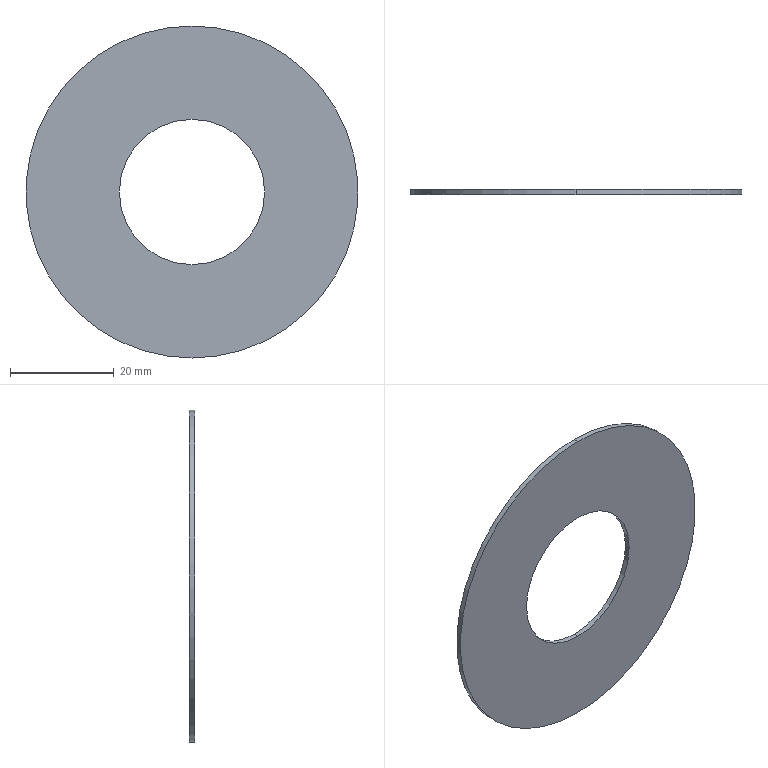Part | STEP file | Emergency Label | 1 solid | 215 faces | box 64 x 1 x 64 mm | volume 2571 mm3 | plane 168 | spline 35 | cylinder 12 | commonest cylinder face diameters 28 x2 33.421 x2 34.221 x2 60.304 x2 61.104 x2 64 x2